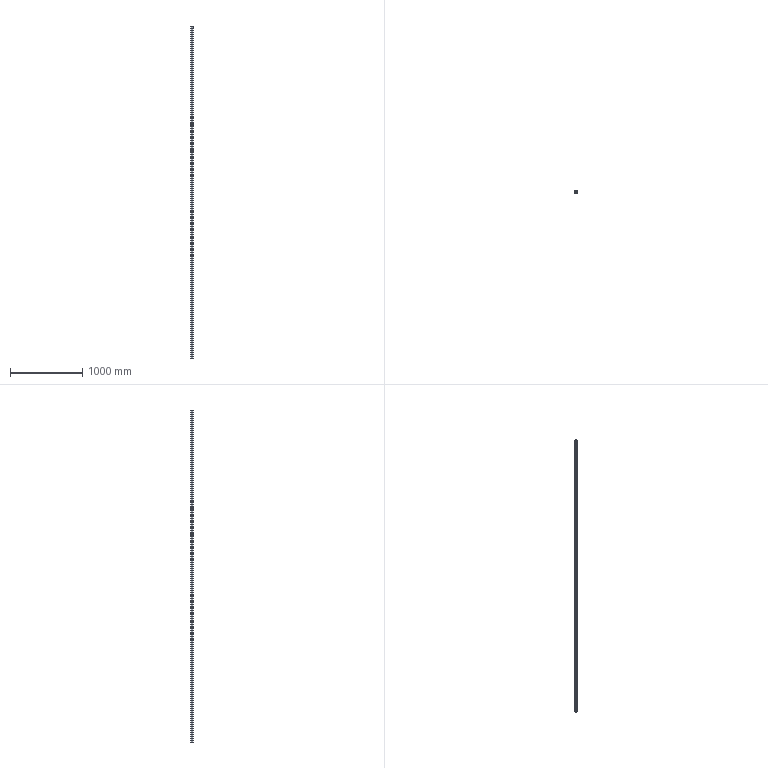Part | NX | features BREP 1 | 1 solid | 46 faces | box 30 x 30 x 4600 mm | volume 1724445 mm3 | plane 33 | cylinder 13 | commonest cylinder face diameters 6 x6 17.968 x5 5 x2